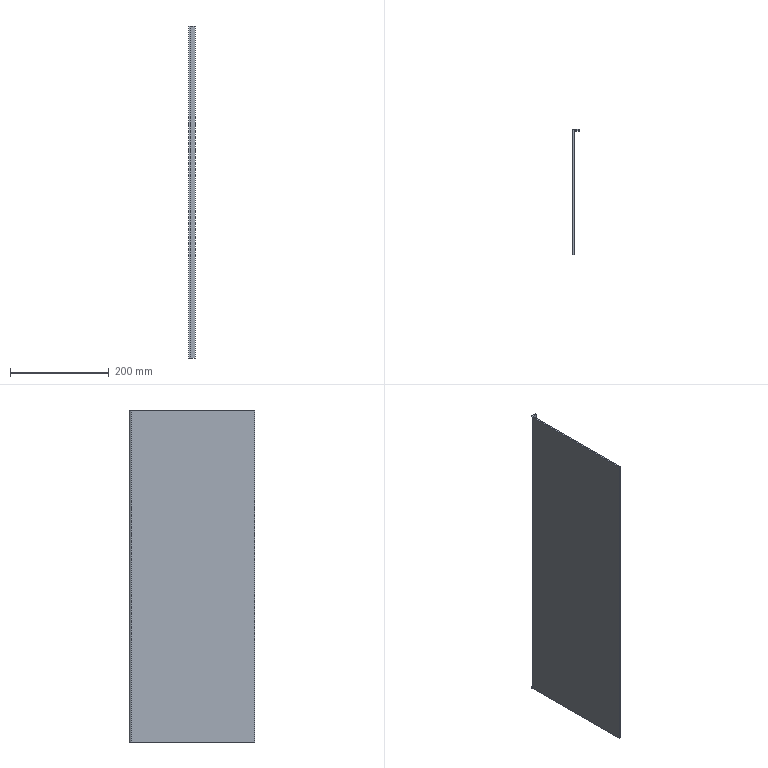Part | STEP file | E3-计量踏Plate 2 | 1 solid | 10 faces | box 14 x 254 x 674 mm | volume 533660 mm3 | plane 8 | cylinder 2 | commonest cylinder face diameters 2 x1 8 x1
STEP:
#1=CARTESIAN_POINT('',(0.,0.,0.));
#2=DIRECTION('',(0.,0.,1.));
#3=DIRECTION('',(1.,0.,0.));
#4=AXIS2_PLACEMENT_3D('',#1,#2,#3);
#5=CARTESIAN_POINT('',(-10.,-3.,337.));
#6=VERTEX_POINT('',#5);
#7=CARTESIAN_POINT('',(0.,-3.,337.));
#8=VERTEX_POINT('',#7);
#9=CARTESIAN_POINT('',(-10.,-3.,337.));
#10=DIRECTION('',(1.,0.,0.));
#11=VECTOR('',#10,1.);
#12=LINE('',#9,#11);
#13=CARTESIAN_POINT('',(-10.,-3.,-337.));
#14=DIRECTION('',(0.,1.,0.));
#15=DIRECTION('',(0.,0.,-1.));
#16=AXIS2_PLACEMENT_3D('',#13,#14,#15);
#17=PLANE('',#16);
#18=CARTESIAN_POINT('',(-674.,0.));
#19=DIRECTION('',(0.,-1.));
#20=VECTOR('',#19,1.);
#21=LINE('',#18,#20);
#22=(GEOMETRIC_REPRESENTATION_CONTEXT(2)PARAMETRIC_REPRESENTATION_CONTEXT()REPRESENTATION_CONTEXT('',''));
#23=DEFINITIONAL_REPRESENTATION('',(#21),#22);
#24=PCURVE('',#17,#23);
#25=CARTESIAN_POINT('',(-10.,-4.,337.));
#26=DIRECTION('',(0.,0.,1.));
#27=DIRECTION('',(-1.,0.,0.));
#28=AXIS2_PLACEMENT_3D('',#25,#26,#27);
#29=PLANE('',#28);
#30=CARTESIAN_POINT('',(0.,-1.));
#31=DIRECTION('',(-1.,0.));
#32=VECTOR('',#31,1.);
#33=LINE('',#30,#32);
#34=(GEOMETRIC_REPRESENTATION_CONTEXT(2)PARAMETRIC_REPRESENTATION_CONTEXT()REPRESENTATION_CONTEXT('',''));
#35=DEFINITIONAL_REPRESENTATION('',(#33),#34);
#36=PCURVE('',#29,#35);
#37=SURFACE_CURVE('',#12,(#24,#36),.PCURVE_S1.);
#38=EDGE_CURVE('',#6,#8,#37,.T.);
#39=ORIENTED_EDGE('',*,*,#38,.F.);
#40=CARTESIAN_POINT('',(-10.,-3.,-337.));
#41=VERTEX_POINT('',#40);
#42=CARTESIAN_POINT('',(-10.,-3.,-337.));
#43=DIRECTION('',(0.,0.,1.));
#44=VECTOR('',#43,1.);
#45=LINE('',#42,#44);
#46=CARTESIAN_POINT('',(0.,0.));
#47=DIRECTION('',(-1.,0.));
#48=VECTOR('',#47,1.);
#49=LINE('',#46,#48);
#50=(GEOMETRIC_REPRESENTATION_CONTEXT(2)PARAMETRIC_REPRESENTATION_CONTEXT()REPRESENTATION_CONTEXT('',''));
#51=DEFINITIONAL_REPRESENTATION('',(#49),#50);
#52=PCURVE('',#17,#51);
#53=CARTESIAN_POINT('',(-10.,-4.,-337.));
#54=DIRECTION('',(0.,0.,1.));
#55=DIRECTION('',(-1.,0.,0.));
#56=AXIS2_PLACEMENT_3D('',#53,#54,#55);
#57=CYLINDRICAL_SURFACE('',#56,1.);
#58=CARTESIAN_POINT('',(4.712,0.));
#59=DIRECTION('',(0.,1.));
#60=VECTOR('',#59,1.);
#61=LINE('',#58,#60);
#62=(GEOMETRIC_REPRESENTATION_CONTEXT(2)PARAMETRIC_REPRESENTATION_CONTEXT()REPRESENTATION_CONTEXT('',''));
#63=DEFINITIONAL_REPRESENTATION('',(#61),#62);
#64=PCURVE('',#57,#63);
#65=SURFACE_CURVE('',#45,(#52,#64),.PCURVE_S1.);
#66=EDGE_CURVE('',#41,#6,#65,.T.);
#67=ORIENTED_EDGE('',*,*,#66,.F.);
#68=CARTESIAN_POINT('',(0.,-3.,-337.));
#69=VERTEX_POINT('',#68);
#70=CARTESIAN_POINT('',(-10.,-3.,-337.));
#71=DIRECTION('',(1.,0.,0.));
#72=VECTOR('',#71,1.);
#73=LINE('',#70,#72);
#74=CARTESIAN_POINT('',(0.,0.));
#75=DIRECTION('',(0.,-1.));
#76=VECTOR('',#75,1.);
#77=LINE('',#74,#76);
#78=(GEOMETRIC_REPRESENTATION_CONTEXT(2)PARAMETRIC_REPRESENTATION_CONTEXT()REPRESENTATION_CONTEXT('',''));
#79=DEFINITIONAL_REPRESENTATION('',(#77),#78);
#80=PCURVE('',#17,#79);
#81=CARTESIAN_POINT('',(-10.,-4.,-337.));
#82=DIRECTION('',(0.,0.,1.));
#83=DIRECTION('',(-1.,0.,0.));
#84=AXIS2_PLACEMENT_3D('',#81,#82,#83);
#85=PLANE('',#84);
#86=CARTESIAN_POINT('',(0.,-1.));
#87=DIRECTION('',(-1.,0.));
#88=VECTOR('',#87,1.);
#89=LINE('',#86,#88);
#90=(GEOMETRIC_REPRESENTATION_CONTEXT(2)PARAMETRIC_REPRESENTATION_CONTEXT()REPRESENTATION_CONTEXT('',''));
#91=DEFINITIONAL_REPRESENTATION('',(#89),#90);
#92=PCURVE('',#85,#91);
#93=SURFACE_CURVE('',#73,(#80,#92),.PCURVE_S1.);
#94=EDGE_CURVE('',#41,#69,#93,.T.);
#95=ORIENTED_EDGE('',*,*,#94,.T.);
#96=CARTESIAN_POINT('',(0.,-3.,-337.));
#97=DIRECTION('',(0.,0.,1.));
#98=VECTOR('',#97,1.);
#99=LINE('',#96,#98);
#100=CARTESIAN_POINT('',(0.,-10.));
#101=DIRECTION('',(-1.,0.));
#102=VECTOR('',#101,1.);
#103=LINE('',#100,#102);
#104=(GEOMETRIC_REPRESENTATION_CONTEXT(2)PARAMETRIC_REPRESENTATION_CONTEXT()REPRESENTATION_CONTEXT('',''));
#105=DEFINITIONAL_REPRESENTATION('',(#103),#104);
#106=PCURVE('',#17,#105);
#107=CARTESIAN_POINT('',(0.,0.,-337.));
#108=DIRECTION('',(1.,0.,0.));
#109=DIRECTION('',(0.,0.,1.));
#110=AXIS2_PLACEMENT_3D('',#107,#108,#109);
#111=PLANE('',#110);
#112=CARTESIAN_POINT('',(0.,3.));
#113=DIRECTION('',(1.,0.));
#114=VECTOR('',#113,1.);
#115=LINE('',#112,#114);
#116=(GEOMETRIC_REPRESENTATION_CONTEXT(2)PARAMETRIC_REPRESENTATION_CONTEXT()REPRESENTATION_CONTEXT('',''));
#117=DEFINITIONAL_REPRESENTATION('',(#115),#116);
#118=PCURVE('',#111,#117);
#119=SURFACE_CURVE('',#99,(#106,#118),.PCURVE_S1.);
#120=EDGE_CURVE('',#69,#8,#119,.T.);
#121=ORIENTED_EDGE('',*,*,#120,.T.);
#122=EDGE_LOOP('',(#39,#67,#95,#121));
#123=FACE_BOUND('',#122,.T.);
#124=ADVANCED_FACE('',(#123),#17,.F.);
#125=CARTESIAN_POINT('',(0.,0.,337.));
#126=VERTEX_POINT('',#125);
#127=CARTESIAN_POINT('',(0.,0.,337.));
#128=DIRECTION('',(0.,-1.,0.));
#129=VECTOR('',#128,1.);
#130=LINE('',#127,#129);
#131=CARTESIAN_POINT('',(674.,0.));
#132=DIRECTION('',(0.,1.));
#133=VECTOR('',#132,1.);
#134=LINE('',#131,#133);
#135=(GEOMETRIC_REPRESENTATION_CONTEXT(2)PARAMETRIC_REPRESENTATION_CONTEXT()REPRESENTATION_CONTEXT('',''));
#136=DEFINITIONAL_REPRESENTATION('',(#134),#135);
#137=PCURVE('',#111,#136);
#138=CARTESIAN_POINT('',(-10.,-4.));
#139=DIRECTION('',(0.,1.));
#140=VECTOR('',#139,1.);
#141=LINE('',#138,#140);
#142=(GEOMETRIC_REPRESENTATION_CONTEXT(2)PARAMETRIC_REPRESENTATION_CONTEXT()REPRESENTATION_CONTEXT('',''));
#143=DEFINITIONAL_REPRESENTATION('',(#141),#142);
#144=PCURVE('',#29,#143);
#145=SURFACE_CURVE('',#130,(#137,#144),.PCURVE_S1.);
#146=EDGE_CURVE('',#126,#8,#145,.T.);
#147=ORIENTED_EDGE('',*,*,#146,.T.);
#148=ORIENTED_EDGE('',*,*,#120,.F.);
#149=CARTESIAN_POINT('',(0.,0.,-337.));
#150=VERTEX_POINT('',#149);
#151=CARTESIAN_POINT('',(0.,0.,-337.));
#152=DIRECTION('',(0.,-1.,0.));
#153=VECTOR('',#152,1.);
#154=LINE('',#151,#153);
#155=CARTESIAN_POINT('',(0.,0.));
#156=DIRECTION('',(0.,1.));
#157=VECTOR('',#156,1.);
#158=LINE('',#155,#157);
#159=(GEOMETRIC_REPRESENTATION_CONTEXT(2)PARAMETRIC_REPRESENTATION_CONTEXT()REPRESENTATION_CONTEXT('',''));
#160=DEFINITIONAL_REPRESENTATION('',(#158),#159);
#161=PCURVE('',#111,#160);
#162=CARTESIAN_POINT('',(-10.,-4.));
#163=DIRECTION('',(0.,1.));
#164=VECTOR('',#163,1.);
#165=LINE('',#162,#164);
#166=(GEOMETRIC_REPRESENTATION_CONTEXT(2)PARAMETRIC_REPRESENTATION_CONTEXT()REPRESENTATION_CONTEXT('',''));
#167=DEFINITIONAL_REPRESENTATION('',(#165),#166);
#168=PCURVE('',#85,#167);
#169=SURFACE_CURVE('',#154,(#161,#168),.PCURVE_S1.);
#170=EDGE_CURVE('',#150,#69,#169,.T.);
#171=ORIENTED_EDGE('',*,*,#170,.F.);
#172=CARTESIAN_POINT('',(0.,0.,-337.));
#173=DIRECTION('',(0.,0.,1.));
#174=VECTOR('',#173,1.);
#175=LINE('',#172,#174);
#176=CARTESIAN_POINT('',(0.,0.));
#177=DIRECTION('',(1.,0.));
#178=VECTOR('',#177,1.);
#179=LINE('',#176,#178);
#180=(GEOMETRIC_REPRESENTATION_CONTEXT(2)PARAMETRIC_REPRESENTATION_CONTEXT()REPRESENTATION_CONTEXT('',''));
#181=DEFINITIONAL_REPRESENTATION('',(#179),#180);
#182=PCURVE('',#111,#181);
#183=CARTESIAN_POINT('',(-10.,0.,-337.));
#184=DIRECTION('',(0.,1.,0.));
#185=DIRECTION('',(0.,0.,-1.));
#186=AXIS2_PLACEMENT_3D('',#183,#184,#185);
#187=PLANE('',#186);
#188=CARTESIAN_POINT('',(0.,-10.));
#189=DIRECTION('',(-1.,0.));
#190=VECTOR('',#189,1.);
#191=LINE('',#188,#190);
#192=(GEOMETRIC_REPRESENTATION_CONTEXT(2)PARAMETRIC_REPRESENTATION_CONTEXT()REPRESENTATION_CONTEXT('',''));
#193=DEFINITIONAL_REPRESENTATION('',(#191),#192);
#194=PCURVE('',#187,#193);
#195=SURFACE_CURVE('',#175,(#182,#194),.PCURVE_S1.);
#196=EDGE_CURVE('',#150,#126,#195,.T.);
#197=ORIENTED_EDGE('',*,*,#196,.T.);
#198=EDGE_LOOP('',(#147,#148,#171,#197));
#199=FACE_BOUND('',#198,.T.);
#200=ADVANCED_FACE('',(#199),#111,.T.);
#201=CARTESIAN_POINT('',(-10.,0.,337.));
#202=VERTEX_POINT('',#201);
#203=CARTESIAN_POINT('',(-10.,0.,337.));
#204=DIRECTION('',(1.,0.,0.));
#205=VECTOR('',#204,1.);
#206=LINE('',#203,#205);
#207=CARTESIAN_POINT('',(-674.,0.));
#208=DIRECTION('',(0.,-1.));
#209=VECTOR('',#208,1.);
#210=LINE('',#207,#209);
#211=(GEOMETRIC_REPRESENTATION_CONTEXT(2)PARAMETRIC_REPRESENTATION_CONTEXT()REPRESENTATION_CONTEXT('',''));
#212=DEFINITIONAL_REPRESENTATION('',(#210),#211);
#213=PCURVE('',#187,#212);
#214=CARTESIAN_POINT('',(0.,-4.));
#215=DIRECTION('',(-1.,0.));
#216=VECTOR('',#215,1.);
#217=LINE('',#214,#216);
#218=(GEOMETRIC_REPRESENTATION_CONTEXT(2)PARAMETRIC_REPRESENTATION_CONTEXT()REPRESENTATION_CONTEXT('',''));
#219=DEFINITIONAL_REPRESENTATION('',(#217),#218);
#220=PCURVE('',#29,#219);
#221=SURFACE_CURVE('',#206,(#213,#220),.PCURVE_S1.);
#222=EDGE_CURVE('',#202,#126,#221,.T.);
#223=ORIENTED_EDGE('',*,*,#222,.T.);
#224=ORIENTED_EDGE('',*,*,#196,.F.);
#225=CARTESIAN_POINT('',(-10.,0.,-337.));
#226=VERTEX_POINT('',#225);
#227=CARTESIAN_POINT('',(-10.,0.,-337.));
#228=DIRECTION('',(1.,0.,0.));
#229=VECTOR('',#228,1.);
#230=LINE('',#227,#229);
#231=CARTESIAN_POINT('',(0.,0.));
#232=DIRECTION('',(0.,-1.));
#233=VECTOR('',#232,1.);
#234=LINE('',#231,#233);
#235=(GEOMETRIC_REPRESENTATION_CONTEXT(2)PARAMETRIC_REPRESENTATION_CONTEXT()REPRESENTATION_CONTEXT('',''));
#236=DEFINITIONAL_REPRESENTATION('',(#234),#235);
#237=PCURVE('',#187,#236);
#238=CARTESIAN_POINT('',(0.,-4.));
#239=DIRECTION('',(-1.,0.));
#240=VECTOR('',#239,1.);
#241=LINE('',#238,#240);
#242=(GEOMETRIC_REPRESENTATION_CONTEXT(2)PARAMETRIC_REPRESENTATION_CONTEXT()REPRESENTATION_CONTEXT('',''));
#243=DEFINITIONAL_REPRESENTATION('',(#241),#242);
#244=PCURVE('',#85,#243);
#245=SURFACE_CURVE('',#230,(#237,#244),.PCURVE_S1.);
#246=EDGE_CURVE('',#226,#150,#245,.T.);
#247=ORIENTED_EDGE('',*,*,#246,.F.);
#248=CARTESIAN_POINT('',(-10.,0.,-337.));
#249=DIRECTION('',(0.,0.,1.));
#250=VECTOR('',#249,1.);
#251=LINE('',#248,#250);
#252=CARTESIAN_POINT('',(0.,0.));
#253=DIRECTION('',(-1.,0.));
#254=VECTOR('',#253,1.);
#255=LINE('',#252,#254);
#256=(GEOMETRIC_REPRESENTATION_CONTEXT(2)PARAMETRIC_REPRESENTATION_CONTEXT()REPRESENTATION_CONTEXT('',''));
#257=DEFINITIONAL_REPRESENTATION('',(#255),#256);
#258=PCURVE('',#187,#257);
#259=CARTESIAN_POINT('',(-10.,-4.,-337.));
#260=DIRECTION('',(0.,0.,1.));
#261=DIRECTION('',(-1.,0.,0.));
#262=AXIS2_PLACEMENT_3D('',#259,#260,#261);
#263=CYLINDRICAL_SURFACE('',#262,4.);
#264=CARTESIAN_POINT('',(4.712,0.));
#265=DIRECTION('',(0.,1.));
#266=VECTOR('',#265,1.);
#267=LINE('',#264,#266);
#268=(GEOMETRIC_REPRESENTATION_CONTEXT(2)PARAMETRIC_REPRESENTATION_CONTEXT()REPRESENTATION_CONTEXT('',''));
#269=DEFINITIONAL_REPRESENTATION('',(#267),#268);
#270=PCURVE('',#263,#269);
#271=SURFACE_CURVE('',#251,(#258,#270),.PCURVE_S1.);
#272=EDGE_CURVE('',#226,#202,#271,.T.);
#273=ORIENTED_EDGE('',*,*,#272,.T.);
#274=EDGE_LOOP('',(#223,#224,#247,#273));
#275=FACE_BOUND('',#274,.T.);
#276=ADVANCED_FACE('',(#275),#187,.T.);
#277=CARTESIAN_POINT('',(-14.,-4.,337.));
#278=VERTEX_POINT('',#277);
#279=CARTESIAN_POINT('',(-10.,-4.,337.));
#280=DIRECTION('',(0.,0.,-1.));
#281=DIRECTION('',(1.,0.,0.));
#282=AXIS2_PLACEMENT_3D('',#279,#280,#281);
#283=CIRCLE('',#282,4.);
#284=CARTESIAN_POINT('',(9.425,674.));
#285=DIRECTION('',(-1.,0.));
#286=VECTOR('',#285,1.);
#287=LINE('',#284,#286);
#288=(GEOMETRIC_REPRESENTATION_CONTEXT(2)PARAMETRIC_REPRESENTATION_CONTEXT()REPRESENTATION_CONTEXT('',''));
#289=DEFINITIONAL_REPRESENTATION('',(#287),#288);
#290=PCURVE('',#263,#289);
#291=CARTESIAN_POINT('',(-4.,0.));
#292=CARTESIAN_POINT('',(-4.,6.928));
#293=CARTESIAN_POINT('',(2.,3.464));
#294=CARTESIAN_POINT('',(8.,0.));
#295=CARTESIAN_POINT('',(2.,-3.464));
#296=CARTESIAN_POINT('',(-4.,-6.928));
#297=CARTESIAN_POINT('',(-4.,0.));
#298=(BOUNDED_CURVE()B_SPLINE_CURVE(2,(#291,#292,#293,#294,#295,#296,#297),.UNSPECIFIED.,.T.,.F.)B_SPLINE_CURVE_WITH_KNOTS((1,2,2,2,2,1),(-2.094,0.,2.094,4.189,6.283,8.378),.UNSPECIFIED.)CURVE()GEOMETRIC_REPRESENTATION_ITEM()RATIONAL_B_SPLINE_CURVE((1.,0.5,1.,0.5,1.,0.5,1.))REPRESENTATION_ITEM(''));
#299=(GEOMETRIC_REPRESENTATION_CONTEXT(2)PARAMETRIC_REPRESENTATION_CONTEXT()REPRESENTATION_CONTEXT('',''));
#300=DEFINITIONAL_REPRESENTATION('',(#298),#299);
#301=PCURVE('',#29,#300);
#302=SURFACE_CURVE('',#283,(#290,#301),.PCURVE_S1.);
#303=EDGE_CURVE('',#278,#202,#302,.T.);
#304=ORIENTED_EDGE('',*,*,#303,.T.);
#305=ORIENTED_EDGE('',*,*,#272,.F.);
#306=CARTESIAN_POINT('',(-14.,-4.,-337.));
#307=VERTEX_POINT('',#306);
#308=CARTESIAN_POINT('',(-10.,-4.,-337.));
#309=DIRECTION('',(0.,0.,-1.));
#310=DIRECTION('',(1.,0.,0.));
#311=AXIS2_PLACEMENT_3D('',#308,#309,#310);
#312=CIRCLE('',#311,4.);
#313=CARTESIAN_POINT('',(9.425,0.));
#314=DIRECTION('',(-1.,0.));
#315=VECTOR('',#314,1.);
#316=LINE('',#313,#315);
#317=(GEOMETRIC_REPRESENTATION_CONTEXT(2)PARAMETRIC_REPRESENTATION_CONTEXT()REPRESENTATION_CONTEXT('',''));
#318=DEFINITIONAL_REPRESENTATION('',(#316),#317);
#319=PCURVE('',#263,#318);
#320=CARTESIAN_POINT('',(-4.,0.));
#321=CARTESIAN_POINT('',(-4.,6.928));
#322=CARTESIAN_POINT('',(2.,3.464));
#323=CARTESIAN_POINT('',(8.,0.));
#324=CARTESIAN_POINT('',(2.,-3.464));
#325=CARTESIAN_POINT('',(-4.,-6.928));
#326=CARTESIAN_POINT('',(-4.,0.));
#327=(BOUNDED_CURVE()B_SPLINE_CURVE(2,(#320,#321,#322,#323,#324,#325,#326),.UNSPECIFIED.,.T.,.F.)B_SPLINE_CURVE_WITH_KNOTS((1,2,2,2,2,1),(-2.094,0.,2.094,4.189,6.283,8.378),.UNSPECIFIED.)CURVE()GEOMETRIC_REPRESENTATION_ITEM()RATIONAL_B_SPLINE_CURVE((1.,0.5,1.,0.5,1.,0.5,1.))REPRESENTATION_ITEM(''));
#328=(GEOMETRIC_REPRESENTATION_CONTEXT(2)PARAMETRIC_REPRESENTATION_CONTEXT()REPRESENTATION_CONTEXT('',''));
#329=DEFINITIONAL_REPRESENTATION('',(#327),#328);
#330=PCURVE('',#85,#329);
#331=SURFACE_CURVE('',#312,(#319,#330),.PCURVE_S1.);
#332=EDGE_CURVE('',#307,#226,#331,.T.);
#333=ORIENTED_EDGE('',*,*,#332,.F.);
#334=CARTESIAN_POINT('',(-14.,-4.,-337.));
#335=DIRECTION('',(0.,0.,1.));
#336=VECTOR('',#335,1.);
#337=LINE('',#334,#336);
#338=CARTESIAN_POINT('',(6.283,0.));
#339=DIRECTION('',(0.,1.));
#340=VECTOR('',#339,1.);
#341=LINE('',#338,#340);
#342=(GEOMETRIC_REPRESENTATION_CONTEXT(2)PARAMETRIC_REPRESENTATION_CONTEXT()REPRESENTATION_CONTEXT('',''));
#343=DEFINITIONAL_REPRESENTATION('',(#341),#342);
#344=PCURVE('',#263,#343);
#345=CARTESIAN_POINT('',(-14.,-4.,-337.));
#346=DIRECTION('',(-1.,0.,0.));
#347=DIRECTION('',(0.,-1.,0.));
#348=AXIS2_PLACEMENT_3D('',#345,#346,#347);
#349=PLANE('',#348);
#350=CARTESIAN_POINT('',(0.,0.));
#351=DIRECTION('',(0.,1.));
#352=VECTOR('',#351,1.);
#353=LINE('',#350,#352);
#354=(GEOMETRIC_REPRESENTATION_CONTEXT(2)PARAMETRIC_REPRESENTATION_CONTEXT()REPRESENTATION_CONTEXT('',''));
#355=DEFINITIONAL_REPRESENTATION('',(#353),#354);
#356=PCURVE('',#349,#355);
#357=SURFACE_CURVE('',#337,(#344,#356),.PCURVE_S1.);
#358=EDGE_CURVE('',#307,#278,#357,.T.);
#359=ORIENTED_EDGE('',*,*,#358,.T.);
#360=EDGE_LOOP('',(#304,#305,#333,#359));
#361=FACE_BOUND('',#360,.T.);
#362=ADVANCED_FACE('',(#361),#263,.T.);
#363=CARTESIAN_POINT('',(-14.,-254.,337.));
#364=VERTEX_POINT('',#363);
#365=CARTESIAN_POINT('',(-14.,-4.,337.));
#366=DIRECTION('',(0.,1.,0.));
#367=VECTOR('',#366,1.);
#368=LINE('',#365,#367);
#369=CARTESIAN_POINT('',(0.,674.));
#370=DIRECTION('',(-1.,0.));
#371=VECTOR('',#370,1.);
#372=LINE('',#369,#371);
#373=(GEOMETRIC_REPRESENTATION_CONTEXT(2)PARAMETRIC_REPRESENTATION_CONTEXT()REPRESENTATION_CONTEXT('',''));
#374=DEFINITIONAL_REPRESENTATION('',(#372),#373);
#375=PCURVE('',#349,#374);
#376=CARTESIAN_POINT('',(4.,0.));
#377=DIRECTION('',(0.,-1.));
#378=VECTOR('',#377,1.);
#379=LINE('',#376,#378);
#380=(GEOMETRIC_REPRESENTATION_CONTEXT(2)PARAMETRIC_REPRESENTATION_CONTEXT()REPRESENTATION_CONTEXT('',''));
#381=DEFINITIONAL_REPRESENTATION('',(#379),#380);
#382=PCURVE('',#29,#381);
#383=SURFACE_CURVE('',#368,(#375,#382),.PCURVE_S1.);
#384=EDGE_CURVE('',#364,#278,#383,.T.);
#385=ORIENTED_EDGE('',*,*,#384,.T.);
#386=ORIENTED_EDGE('',*,*,#358,.F.);
#387=CARTESIAN_POINT('',(-14.,-254.,-337.));
#388=VERTEX_POINT('',#387);
#389=CARTESIAN_POINT('',(-14.,-4.,-337.));
#390=DIRECTION('',(0.,1.,0.));
#391=VECTOR('',#390,1.);
#392=LINE('',#389,#391);
#393=CARTESIAN_POINT('',(0.,0.));
#394=DIRECTION('',(-1.,0.));
#395=VECTOR('',#394,1.);
#396=LINE('',#393,#395);
#397=(GEOMETRIC_REPRESENTATION_CONTEXT(2)PARAMETRIC_REPRESENTATION_CONTEXT()REPRESENTATION_CONTEXT('',''));
#398=DEFINITIONAL_REPRESENTATION('',(#396),#397);
#399=PCURVE('',#349,#398);
#400=CARTESIAN_POINT('',(4.,0.));
#401=DIRECTION('',(0.,-1.));
#402=VECTOR('',#401,1.);
#403=LINE('',#400,#402);
#404=(GEOMETRIC_REPRESENTATION_CONTEXT(2)PARAMETRIC_REPRESENTATION_CONTEXT()REPRESENTATION_CONTEXT('',''));
#405=DEFINITIONAL_REPRESENTATION('',(#403),#404);
#406=PCURVE('',#85,#405);
#407=SURFACE_CURVE('',#392,(#399,#406),.PCURVE_S1.);
#408=EDGE_CURVE('',#388,#307,#407,.T.);
#409=ORIENTED_EDGE('',*,*,#408,.F.);
#410=CARTESIAN_POINT('',(-14.,-254.,-337.));
#411=DIRECTION('',(0.,0.,1.));
#412=VECTOR('',#411,1.);
#413=LINE('',#410,#412);
#414=CARTESIAN_POINT('',(250.,0.));
#415=DIRECTION('',(0.,1.));
#416=VECTOR('',#415,1.);
#417=LINE('',#414,#416);
#418=(GEOMETRIC_REPRESENTATION_CONTEXT(2)PARAMETRIC_REPRESENTATION_CONTEXT()REPRESENTATION_CONTEXT('',''));
#419=DEFINITIONAL_REPRESENTATION('',(#417),#418);
#420=PCURVE('',#349,#419);
#421=CARTESIAN_POINT('',(-11.,-254.,-337.));
#422=DIRECTION('',(0.,-1.,0.));
#423=DIRECTION('',(0.,0.,1.));
#424=AXIS2_PLACEMENT_3D('',#421,#422,#423);
#425=PLANE('',#424);
#426=CARTESIAN_POINT('',(0.,3.));
#427=DIRECTION('',(1.,0.));
#428=VECTOR('',#427,1.);
#429=LINE('',#426,#428);
#430=(GEOMETRIC_REPRESENTATION_CONTEXT(2)PARAMETRIC_REPRESENTATION_CONTEXT()REPRESENTATION_CONTEXT('',''));
#431=DEFINITIONAL_REPRESENTATION('',(#429),#430);
#432=PCURVE('',#425,#431);
#433=SURFACE_CURVE('',#413,(#420,#432),.PCURVE_S1.);
#434=EDGE_CURVE('',#388,#364,#433,.T.);
#435=ORIENTED_EDGE('',*,*,#434,.T.);
#436=EDGE_LOOP('',(#385,#386,#409,#435));
#437=FACE_BOUND('',#436,.T.);
#438=ADVANCED_FACE('',(#437),#349,.T.);
#439=CARTESIAN_POINT('',(-11.,-254.,337.));
#440=VERTEX_POINT('',#439);
#441=CARTESIAN_POINT('',(-11.,-254.,337.));
#442=DIRECTION('',(-1.,0.,0.));
#443=VECTOR('',#442,1.);
#444=LINE('',#441,#443);
#445=CARTESIAN_POINT('',(674.,0.));
#446=DIRECTION('',(0.,1.));
#447=VECTOR('',#446,1.);
#448=LINE('',#445,#447);
#449=(GEOMETRIC_REPRESENTATION_CONTEXT(2)PARAMETRIC_REPRESENTATION_CONTEXT()REPRESENTATION_CONTEXT('',''));
#450=DEFINITIONAL_REPRESENTATION('',(#448),#449);
#451=PCURVE('',#425,#450);
#452=CARTESIAN_POINT('',(1.,250.));
#453=DIRECTION('',(1.,0.));
#454=VECTOR('',#453,1.);
#455=LINE('',#452,#454);
#456=(GEOMETRIC_REPRESENTATION_CONTEXT(2)PARAMETRIC_REPRESENTATION_CONTEXT()REPRESENTATION_CONTEXT('',''));
#457=DEFINITIONAL_REPRESENTATION('',(#455),#456);
#458=PCURVE('',#29,#457);
#459=SURFACE_CURVE('',#444,(#451,#458),.PCURVE_S1.);
#460=EDGE_CURVE('',#440,#364,#459,.T.);
#461=ORIENTED_EDGE('',*,*,#460,.T.);
#462=ORIENTED_EDGE('',*,*,#434,.F.);
#463=CARTESIAN_POINT('',(-11.,-254.,-337.));
#464=VERTEX_POINT('',#463);
#465=CARTESIAN_POINT('',(-11.,-254.,-337.));
#466=DIRECTION('',(-1.,0.,0.));
#467=VECTOR('',#466,1.);
#468=LINE('',#465,#467);
#469=CARTESIAN_POINT('',(0.,0.));
#470=DIRECTION('',(0.,1.));
#471=VECTOR('',#470,1.);
#472=LINE('',#469,#471);
#473=(GEOMETRIC_REPRESENTATION_CONTEXT(2)PARAMETRIC_REPRESENTATION_CONTEXT()REPRESENTATION_CONTEXT('',''));
#474=DEFINITIONAL_REPRESENTATION('',(#472),#473);
#475=PCURVE('',#425,#474);
#476=CARTESIAN_POINT('',(1.,250.));
#477=DIRECTION('',(1.,0.));
#478=VECTOR('',#477,1.);
#479=LINE('',#476,#478);
#480=(GEOMETRIC_REPRESENTATION_CONTEXT(2)PARAMETRIC_REPRESENTATION_CONTEXT()REPRESENTATION_CONTEXT('',''));
#481=DEFINITIONAL_REPRESENTATION('',(#479),#480);
#482=PCURVE('',#85,#481);
#483=SURFACE_CURVE('',#468,(#475,#482),.PCURVE_S1.);
#484=EDGE_CURVE('',#464,#388,#483,.T.);
#485=ORIENTED_EDGE('',*,*,#484,.F.);
#486=CARTESIAN_POINT('',(-11.,-254.,-337.));
#487=DIRECTION('',(0.,0.,1.));
#488=VECTOR('',#487,1.);
#489=LINE('',#486,#488);
#490=CARTESIAN_POINT('',(0.,0.));
#491=DIRECTION('',(1.,0.));
#492=VECTOR('',#491,1.);
#493=LINE('',#490,#492);
#494=(GEOMETRIC_REPRESENTATION_CONTEXT(2)PARAMETRIC_REPRESENTATION_CONTEXT()REPRESENTATION_CONTEXT('',''));
#495=DEFINITIONAL_REPRESENTATION('',(#493),#494);
#496=PCURVE('',#425,#495);
#497=CARTESIAN_POINT('',(-11.,-4.,-337.));
#498=DIRECTION('',(-1.,0.,0.));
#499=DIRECTION('',(0.,-1.,0.));
#500=AXIS2_PLACEMENT_3D('',#497,#498,#499);
#501=PLANE('',#500);
#502=CARTESIAN_POINT('',(250.,0.));
#503=DIRECTION('',(0.,1.));
#504=VECTOR('',#503,1.);
#505=LINE('',#502,#504);
#506=(GEOMETRIC_REPRESENTATION_CONTEXT(2)PARAMETRIC_REPRESENTATION_CONTEXT()REPRESENTATION_CONTEXT('',''));
#507=DEFINITIONAL_REPRESENTATION('',(#505),#506);
#508=PCURVE('',#501,#507);
#509=SURFACE_CURVE('',#489,(#496,#508),.PCURVE_S1.);
#510=EDGE_CURVE('',#464,#440,#509,.T.);
#511=ORIENTED_EDGE('',*,*,#510,.T.);
#512=EDGE_LOOP('',(#461,#462,#485,#511));
#513=FACE_BOUND('',#512,.T.);
#514=ADVANCED_FACE('',(#513),#425,.T.);
#515=CARTESIAN_POINT('',(-11.,-4.,337.));
#516=VERTEX_POINT('',#515);
#517=CARTESIAN_POINT('',(-11.,-4.,337.));
#518=DIRECTION('',(0.,1.,0.));
#519=VECTOR('',#518,1.);
#520=LINE('',#517,#519);
#521=CARTESIAN_POINT('',(0.,674.));
#522=DIRECTION('',(-1.,0.));
#523=VECTOR('',#522,1.);
#524=LINE('',#521,#523);
#525=(GEOMETRIC_REPRESENTATION_CONTEXT(2)PARAMETRIC_REPRESENTATION_CONTEXT()REPRESENTATION_CONTEXT('',''));
#526=DEFINITIONAL_REPRESENTATION('',(#524),#525);
#527=PCURVE('',#501,#526);
#528=CARTESIAN_POINT('',(1.,0.));
#529=DIRECTION('',(0.,-1.));
#530=VECTOR('',#529,1.);
#531=LINE('',#528,#530);
#532=(GEOMETRIC_REPRESENTATION_CONTEXT(2)PARAMETRIC_REPRESENTATION_CONTEXT()REPRESENTATION_CONTEXT('',''));
#533=DEFINITIONAL_REPRESENTATION('',(#531),#532);
#534=PCURVE('',#29,#533);
#535=SURFACE_CURVE('',#520,(#527,#534),.PCURVE_S1.);
#536=EDGE_CURVE('',#440,#516,#535,.T.);
#537=ORIENTED_EDGE('',*,*,#536,.F.);
#538=ORIENTED_EDGE('',*,*,#510,.F.);
#539=CARTESIAN_POINT('',(-11.,-4.,-337.));
#540=VERTEX_POINT('',#539);
#541=CARTESIAN_POINT('',(-11.,-4.,-337.));
#542=DIRECTION('',(0.,1.,0.));
#543=VECTOR('',#542,1.);
#544=LINE('',#541,#543);
#545=CARTESIAN_POINT('',(0.,0.));
#546=DIRECTION('',(-1.,0.));
#547=VECTOR('',#546,1.);
#548=LINE('',#545,#547);
#549=(GEOMETRIC_REPRESENTATION_CONTEXT(2)PARAMETRIC_REPRESENTATION_CONTEXT()REPRESENTATION_CONTEXT('',''));
#550=DEFINITIONAL_REPRESENTATION('',(#548),#549);
#551=PCURVE('',#501,#550);
#552=CARTESIAN_POINT('',(1.,0.));
#553=DIRECTION('',(0.,-1.));
#554=VECTOR('',#553,1.);
#555=LINE('',#552,#554);
#556=(GEOMETRIC_REPRESENTATION_CONTEXT(2)PARAMETRIC_REPRESENTATION_CONTEXT()REPRESENTATION_CONTEXT('',''));
#557=DEFINITIONAL_REPRESENTATION('',(#555),#556);
#558=PCURVE('',#85,#557);
#559=SURFACE_CURVE('',#544,(#551,#558),.PCURVE_S1.);
#560=EDGE_CURVE('',#464,#540,#559,.T.);
#561=ORIENTED_EDGE('',*,*,#560,.T.);
#562=CARTESIAN_POINT('',(-11.,-4.,-337.));
#563=DIRECTION('',(0.,0.,1.));
#564=VECTOR('',#563,1.);
#565=LINE('',#562,#564);
#566=CARTESIAN_POINT('',(0.,0.));
#567=DIRECTION('',(0.,1.));
#568=VECTOR('',#567,1.);
#569=LINE('',#566,#568);
#570=(GEOMETRIC_REPRESENTATION_CONTEXT(2)PARAMETRIC_REPRESENTATION_CONTEXT()REPRESENTATION_CONTEXT('',''));
#571=DEFINITIONAL_REPRESENTATION('',(#569),#570);
#572=PCURVE('',#501,#571);
#573=CARTESIAN_POINT('',(6.283,0.));
#574=DIRECTION('',(0.,1.));
#575=VECTOR('',#574,1.);
#576=LINE('',#573,#575);
#577=(GEOMETRIC_REPRESENTATION_CONTEXT(2)PARAMETRIC_REPRESENTATION_CONTEXT()REPRESENTATION_CONTEXT('',''));
#578=DEFINITIONAL_REPRESENTATION('',(#576),#577);
#579=PCURVE('',#57,#578);
#580=SURFACE_CURVE('',#565,(#572,#579),.PCURVE_S1.);
#581=EDGE_CURVE('',#540,#516,#580,.T.);
#582=ORIENTED_EDGE('',*,*,#581,.T.);
#583=EDGE_LOOP('',(#537,#538,#561,#582));
#584=FACE_BOUND('',#583,.T.);
#585=ADVANCED_FACE('',(#584),#501,.F.);
#586=ORIENTED_EDGE('',*,*,#66,.F.);
#587=CARTESIAN_POINT('',(-10.,-4.,-337.));
#588=DIRECTION('',(0.,0.,-1.));
#589=DIRECTION('',(1.,0.,0.));
#590=AXIS2_PLACEMENT_3D('',#587,#588,#589);
#591=CIRCLE('',#590,1.);
#592=CARTESIAN_POINT('',(9.425,0.));
#593=DIRECTION('',(-1.,0.));
#594=VECTOR('',#593,1.);
#595=LINE('',#592,#594);
#596=(GEOMETRIC_REPRESENTATION_CONTEXT(2)PARAMETRIC_REPRESENTATION_CONTEXT()REPRESENTATION_CONTEXT('',''));
#597=DEFINITIONAL_REPRESENTATION('',(#595),#596);
#598=PCURVE('',#57,#597);
#599=CARTESIAN_POINT('',(-1.,0.));
#600=CARTESIAN_POINT('',(-1.,1.732));
#601=CARTESIAN_POINT('',(0.5,0.866));
#602=CARTESIAN_POINT('',(2.,0.));
#603=CARTESIAN_POINT('',(0.5,-0.866));
#604=CARTESIAN_POINT('',(-1.,-1.732));
#605=CARTESIAN_POINT('',(-1.,0.));
#606=(BOUNDED_CURVE()B_SPLINE_CURVE(2,(#599,#600,#601,#602,#603,#604,#605),.UNSPECIFIED.,.T.,.F.)B_SPLINE_CURVE_WITH_KNOTS((1,2,2,2,2,1),(-2.094,0.,2.094,4.189,6.283,8.378),.UNSPECIFIED.)CURVE()GEOMETRIC_REPRESENTATION_ITEM()RATIONAL_B_SPLINE_CURVE((1.,0.5,1.,0.5,1.,0.5,1.))REPRESENTATION_ITEM(''));
#607=(GEOMETRIC_REPRESENTATION_CONTEXT(2)PARAMETRIC_REPRESENTATION_CONTEXT()REPRESENTATION_CONTEXT('',''));
#608=DEFINITIONAL_REPRESENTATION('',(#606),#607);
#609=PCURVE('',#85,#608);
#610=SURFACE_CURVE('',#591,(#598,#609),.PCURVE_S1.);
#611=EDGE_CURVE('',#540,#41,#610,.T.);
#612=ORIENTED_EDGE('',*,*,#611,.F.);
#613=ORIENTED_EDGE('',*,*,#581,.T.);
#614=CARTESIAN_POINT('',(-10.,-4.,337.));
#615=DIRECTION('',(0.,0.,-1.));
#616=DIRECTION('',(1.,0.,0.));
#617=AXIS2_PLACEMENT_3D('',#614,#615,#616);
#618=CIRCLE('',#617,1.);
#619=CARTESIAN_POINT('',(9.425,674.));
#620=DIRECTION('',(-1.,0.));
#621=VECTOR('',#620,1.);
#622=LINE('',#619,#621);
#623=(GEOMETRIC_REPRESENTATION_CONTEXT(2)PARAMETRIC_REPRESENTATION_CONTEXT()REPRESENTATION_CONTEXT('',''));
#624=DEFINITIONAL_REPRESENTATION('',(#622),#623);
#625=PCURVE('',#57,#624);
#626=CARTESIAN_POINT('',(-1.,0.));
#627=CARTESIAN_POINT('',(-1.,1.732));
#628=CARTESIAN_POINT('',(0.5,0.866));
#629=CARTESIAN_POINT('',(2.,0.));
#630=CARTESIAN_POINT('',(0.5,-0.866));
#631=CARTESIAN_POINT('',(-1.,-1.732));
#632=CARTESIAN_POINT('',(-1.,0.));
#633=(BOUNDED_CURVE()B_SPLINE_CURVE(2,(#626,#627,#628,#629,#630,#631,#632),.UNSPECIFIED.,.T.,.F.)B_SPLINE_CURVE_WITH_KNOTS((1,2,2,2,2,1),(-2.094,0.,2.094,4.189,6.283,8.378),.UNSPECIFIED.)CURVE()GEOMETRIC_REPRESENTATION_ITEM()RATIONAL_B_SPLINE_CURVE((1.,0.5,1.,0.5,1.,0.5,1.))REPRESENTATION_ITEM(''));
#634=(GEOMETRIC_REPRESENTATION_CONTEXT(2)PARAMETRIC_REPRESENTATION_CONTEXT()REPRESENTATION_CONTEXT('',''));
#635=DEFINITIONAL_REPRESENTATION('',(#633),#634);
#636=PCURVE('',#29,#635);
#637=SURFACE_CURVE('',#618,(#625,#636),.PCURVE_S1.);
#638=EDGE_CURVE('',#516,#6,#637,.T.);
#639=ORIENTED_EDGE('',*,*,#638,.T.);
#640=EDGE_LOOP('',(#586,#612,#613,#639));
#641=FACE_BOUND('',#640,.F.);
#642=ADVANCED_FACE('',(#641),#57,.F.);
#643=ORIENTED_EDGE('',*,*,#94,.F.);
#644=ORIENTED_EDGE('',*,*,#611,.F.);
#645=ORIENTED_EDGE('',*,*,#560,.F.);
#646=ORIENTED_EDGE('',*,*,#484,.T.);
#647=ORIENTED_EDGE('',*,*,#408,.T.);
#648=ORIENTED_EDGE('',*,*,#332,.T.);
#649=ORIENTED_EDGE('',*,*,#246,.T.);
#650=ORIENTED_EDGE('',*,*,#170,.T.);
#651=EDGE_LOOP('',(#643,#644,#645,#646,#647,#648,#649,#650));
#652=FACE_BOUND('',#651,.T.);
#653=ADVANCED_FACE('',(#652),#85,.F.);
#654=ORIENTED_EDGE('',*,*,#38,.T.);
#655=ORIENTED_EDGE('',*,*,#146,.F.);
#656=ORIENTED_EDGE('',*,*,#222,.F.);
#657=ORIENTED_EDGE('',*,*,#303,.F.);
#658=ORIENTED_EDGE('',*,*,#384,.F.);
#659=ORIENTED_EDGE('',*,*,#460,.F.);
#660=ORIENTED_EDGE('',*,*,#536,.T.);
#661=ORIENTED_EDGE('',*,*,#638,.T.);
#662=EDGE_LOOP('',(#654,#655,#656,#657,#658,#659,#660,#661));
#663=FACE_BOUND('',#662,.T.);
#664=ADVANCED_FACE('',(#663),#29,.T.);
#665=CLOSED_SHELL('',(#124,#200,#276,#362,#438,#514,#585,#642,#653,#664));
#666=MANIFOLD_SOLID_BREP('',#665);
#667=(LENGTH_UNIT()NAMED_UNIT(*)SI_UNIT(.MILLI.,.METRE.));
#668=UNCERTAINTY_MEASURE_WITH_UNIT(LENGTH_MEASURE(0.0000001),#667,'','');
#669=(NAMED_UNIT(*)PLANE_ANGLE_UNIT()SI_UNIT($,.RADIAN.));
#670=(NAMED_UNIT(*)SI_UNIT($,.STERADIAN.)SOLID_ANGLE_UNIT());
#671=(GEOMETRIC_REPRESENTATION_CONTEXT(3)GLOBAL_UNCERTAINTY_ASSIGNED_CONTEXT((#668))GLOBAL_UNIT_ASSIGNED_CONTEXT((#667,#669,#670))REPRESENTATION_CONTEXT('',''));
#672=ADVANCED_BREP_SHAPE_REPRESENTATION('',(#4,#666),#671);